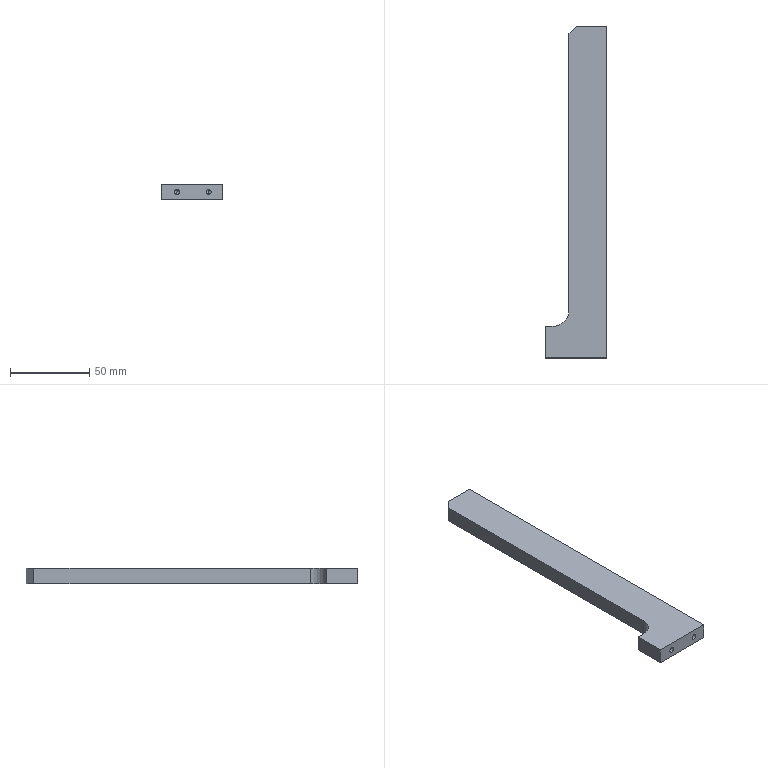Part | STEP file | 0243_207_Rib | 1 solid | 30 faces | box 39 x 210 x 10 mm | volume 52975 mm3 | cylinder 11 | cone 10 | plane 9 | commonest cylinder face diameters 3.3 x10 20 x1